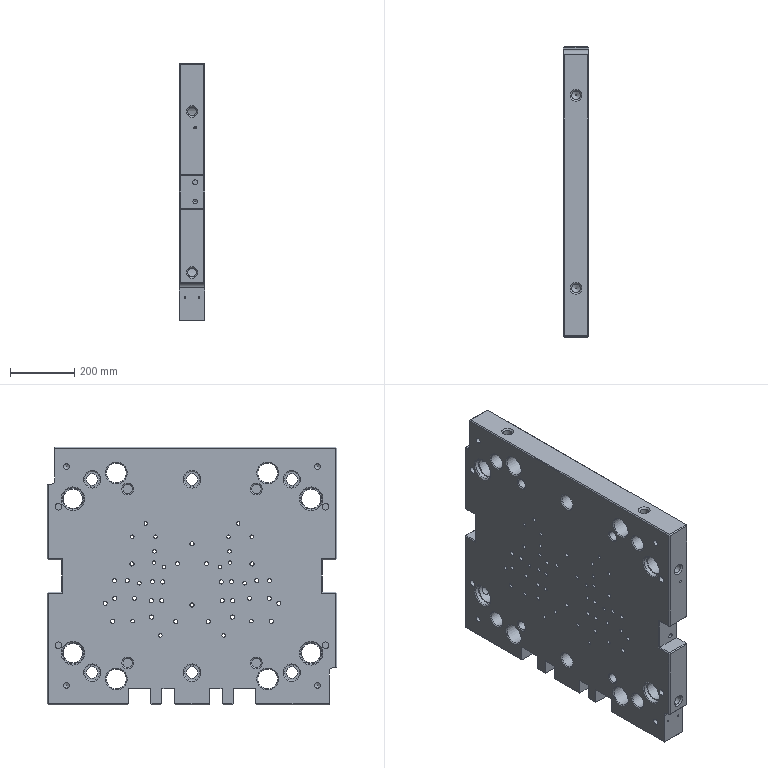Part | STEP file | solid 142 | 1 solid | 356 faces | box 80 x 900 x 800 mm | volume 51885032 mm3 | plane 164 | cylinder 124 | cone 68 | commonest cylinder face diameters 13 x30 11 x18 16 x12 14 x10 26.5 x6 30 x6